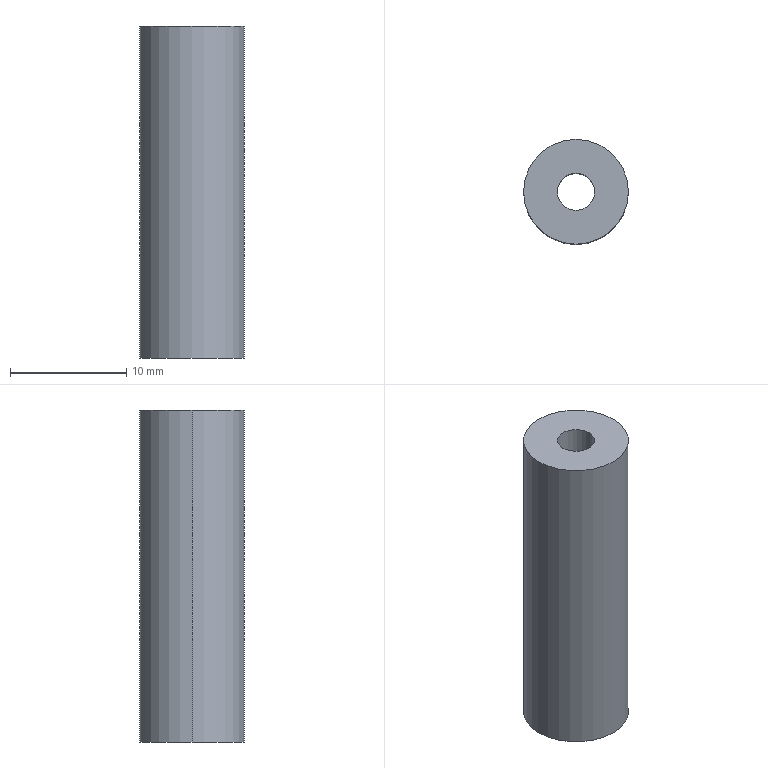Part | SolidWorks | features Extrusion 1 | 1 solid | 6 faces | box 9 x 9 x 28.5 mm | volume 1584 mm3 | cylinder 4 | plane 2 | commonest cylinder face diameters 3.2 x2 9 x2
STEP:
#1=CARTESIAN_POINT('',(-1.6,0.,14.25));
#2=VERTEX_POINT('',#1);
#3=CARTESIAN_POINT('',(1.6,0.,14.25));
#4=VERTEX_POINT('',#3);
#5=CARTESIAN_POINT('',(0.,0.,14.25));
#6=DIRECTION('',(0.,0.,1.));
#7=DIRECTION('',(1.,0.,0.));
#8=AXIS2_PLACEMENT_3D('',#5,#6,#7);
#9=CIRCLE('',#8,1.6);
#10=EDGE_CURVE('',#2,#4,#9,.T.);
#11=ORIENTED_EDGE('',*,*,#10,.T.);
#12=CARTESIAN_POINT('',(1.6,0.,-14.25));
#13=VERTEX_POINT('',#12);
#14=CARTESIAN_POINT('',(1.6,0.,14.25));
#15=DIRECTION('',(0.,0.,-1.));
#16=VECTOR('',#15,1000.);
#17=LINE('',#14,#16);
#18=EDGE_CURVE('',#4,#13,#17,.T.);
#19=ORIENTED_EDGE('',*,*,#18,.T.);
#20=CARTESIAN_POINT('',(-1.6,0.,-14.25));
#21=VERTEX_POINT('',#20);
#22=CARTESIAN_POINT('',(0.,0.,-14.25));
#23=DIRECTION('',(0.,0.,1.));
#24=DIRECTION('',(1.,0.,0.));
#25=AXIS2_PLACEMENT_3D('',#22,#23,#24);
#26=CIRCLE('',#25,1.6);
#27=EDGE_CURVE('',#21,#13,#26,.T.);
#28=ORIENTED_EDGE('',*,*,#27,.F.);
#29=CARTESIAN_POINT('',(-1.6,0.,14.25));
#30=DIRECTION('',(0.,0.,-1.));
#31=VECTOR('',#30,1000.);
#32=LINE('',#29,#31);
#33=EDGE_CURVE('',#2,#21,#32,.T.);
#34=ORIENTED_EDGE('',*,*,#33,.F.);
#35=EDGE_LOOP('',(#11,#19,#28,#34));
#36=FACE_OUTER_BOUND('',#35,.T.);
#37=CARTESIAN_POINT('',(0.,0.,14.25));
#38=DIRECTION('',(0.,0.,-1.));
#39=DIRECTION('',(-1.,0.,0.));
#40=AXIS2_PLACEMENT_3D('',#37,#38,#39);
#41=CYLINDRICAL_SURFACE('',#40,1.6);
#42=ADVANCED_FACE('',(#36),#41,.F.);
#43=CARTESIAN_POINT('',(4.5,0.,14.25));
#44=VERTEX_POINT('',#43);
#45=CARTESIAN_POINT('',(-4.5,0.,14.25));
#46=VERTEX_POINT('',#45);
#47=CARTESIAN_POINT('',(0.,0.,14.25));
#48=DIRECTION('',(0.,0.,1.));
#49=DIRECTION('',(1.,0.,0.));
#50=AXIS2_PLACEMENT_3D('',#47,#48,#49);
#51=CIRCLE('',#50,4.5);
#52=EDGE_CURVE('',#44,#46,#51,.T.);
#53=ORIENTED_EDGE('',*,*,#52,.F.);
#54=CARTESIAN_POINT('',(4.5,0.,-14.25));
#55=VERTEX_POINT('',#54);
#56=CARTESIAN_POINT('',(4.5,0.,14.25));
#57=DIRECTION('',(0.,0.,-1.));
#58=VECTOR('',#57,1000.);
#59=LINE('',#56,#58);
#60=EDGE_CURVE('',#44,#55,#59,.T.);
#61=ORIENTED_EDGE('',*,*,#60,.T.);
#62=CARTESIAN_POINT('',(-4.5,0.,-14.25));
#63=VERTEX_POINT('',#62);
#64=CARTESIAN_POINT('',(0.,0.,-14.25));
#65=DIRECTION('',(0.,0.,1.));
#66=DIRECTION('',(1.,0.,0.));
#67=AXIS2_PLACEMENT_3D('',#64,#65,#66);
#68=CIRCLE('',#67,4.5);
#69=EDGE_CURVE('',#55,#63,#68,.T.);
#70=ORIENTED_EDGE('',*,*,#69,.T.);
#71=CARTESIAN_POINT('',(-4.5,0.,14.25));
#72=DIRECTION('',(0.,0.,-1.));
#73=VECTOR('',#72,1000.);
#74=LINE('',#71,#73);
#75=EDGE_CURVE('',#46,#63,#74,.T.);
#76=ORIENTED_EDGE('',*,*,#75,.F.);
#77=EDGE_LOOP('',(#53,#61,#70,#76));
#78=FACE_OUTER_BOUND('',#77,.T.);
#79=CARTESIAN_POINT('',(0.,0.,14.25));
#80=DIRECTION('',(0.,0.,-1.));
#81=DIRECTION('',(-1.,0.,0.));
#82=AXIS2_PLACEMENT_3D('',#79,#80,#81);
#83=CYLINDRICAL_SURFACE('',#82,4.5);
#84=ADVANCED_FACE('',(#78),#83,.T.);
#85=CARTESIAN_POINT('',(0.,0.,14.25));
#86=DIRECTION('',(0.,0.,1.));
#87=DIRECTION('',(1.,0.,0.));
#88=AXIS2_PLACEMENT_3D('',#85,#86,#87);
#89=CIRCLE('',#88,4.5);
#90=EDGE_CURVE('',#46,#44,#89,.T.);
#91=ORIENTED_EDGE('',*,*,#90,.T.);
#92=ORIENTED_EDGE('',*,*,#52,.T.);
#93=EDGE_LOOP('',(#91,#92));
#94=FACE_OUTER_BOUND('',#93,.T.);
#95=ORIENTED_EDGE('',*,*,#10,.F.);
#96=CARTESIAN_POINT('',(0.,0.,14.25));
#97=DIRECTION('',(0.,0.,1.));
#98=DIRECTION('',(1.,0.,0.));
#99=AXIS2_PLACEMENT_3D('',#96,#97,#98);
#100=CIRCLE('',#99,1.6);
#101=EDGE_CURVE('',#4,#2,#100,.T.);
#102=ORIENTED_EDGE('',*,*,#101,.F.);
#103=EDGE_LOOP('',(#95,#102));
#104=FACE_BOUND('',#103,.T.);
#105=CARTESIAN_POINT('',(0.,0.,14.25));
#106=DIRECTION('',(0.,0.,1.));
#107=DIRECTION('',(1.,0.,0.));
#108=AXIS2_PLACEMENT_3D('',#105,#106,#107);
#109=PLANE('',#108);
#110=ADVANCED_FACE('',(#94,#104),#109,.T.);
#111=CARTESIAN_POINT('',(0.,0.,-14.25));
#112=DIRECTION('',(0.,0.,1.));
#113=DIRECTION('',(1.,0.,0.));
#114=AXIS2_PLACEMENT_3D('',#111,#112,#113);
#115=CIRCLE('',#114,4.5);
#116=EDGE_CURVE('',#63,#55,#115,.T.);
#117=ORIENTED_EDGE('',*,*,#116,.F.);
#118=ORIENTED_EDGE('',*,*,#69,.F.);
#119=EDGE_LOOP('',(#117,#118));
#120=FACE_OUTER_BOUND('',#119,.T.);
#121=ORIENTED_EDGE('',*,*,#27,.T.);
#122=CARTESIAN_POINT('',(0.,0.,-14.25));
#123=DIRECTION('',(0.,0.,1.));
#124=DIRECTION('',(1.,0.,0.));
#125=AXIS2_PLACEMENT_3D('',#122,#123,#124);
#126=CIRCLE('',#125,1.6);
#127=EDGE_CURVE('',#13,#21,#126,.T.);
#128=ORIENTED_EDGE('',*,*,#127,.T.);
#129=EDGE_LOOP('',(#121,#128));
#130=FACE_BOUND('',#129,.T.);
#131=CARTESIAN_POINT('',(0.,0.,-14.25));
#132=DIRECTION('',(0.,0.,1.));
#133=DIRECTION('',(1.,0.,0.));
#134=AXIS2_PLACEMENT_3D('',#131,#132,#133);
#135=PLANE('',#134);
#136=ADVANCED_FACE('',(#120,#130),#135,.F.);
#137=ORIENTED_EDGE('',*,*,#60,.F.);
#138=ORIENTED_EDGE('',*,*,#90,.F.);
#139=ORIENTED_EDGE('',*,*,#75,.T.);
#140=ORIENTED_EDGE('',*,*,#116,.T.);
#141=EDGE_LOOP('',(#137,#138,#139,#140));
#142=FACE_OUTER_BOUND('',#141,.T.);
#143=CARTESIAN_POINT('',(0.,0.,14.25));
#144=DIRECTION('',(0.,0.,-1.));
#145=DIRECTION('',(-1.,0.,0.));
#146=AXIS2_PLACEMENT_3D('',#143,#144,#145);
#147=CYLINDRICAL_SURFACE('',#146,4.5);
#148=ADVANCED_FACE('',(#142),#147,.T.);
#149=ORIENTED_EDGE('',*,*,#18,.F.);
#150=ORIENTED_EDGE('',*,*,#101,.T.);
#151=ORIENTED_EDGE('',*,*,#33,.T.);
#152=ORIENTED_EDGE('',*,*,#127,.F.);
#153=EDGE_LOOP('',(#149,#150,#151,#152));
#154=FACE_OUTER_BOUND('',#153,.T.);
#155=CARTESIAN_POINT('',(0.,0.,14.25));
#156=DIRECTION('',(0.,0.,-1.));
#157=DIRECTION('',(-1.,0.,0.));
#158=AXIS2_PLACEMENT_3D('',#155,#156,#157);
#159=CYLINDRICAL_SURFACE('',#158,1.6);
#160=ADVANCED_FACE('',(#154),#159,.F.);
#161=CLOSED_SHELL('',(#42,#84,#110,#136,#148,#160));
#162=MANIFOLD_SOLID_BREP('',#161);
#163=CARTESIAN_POINT('',(0.,0.,0.));
#164=DIRECTION('',(0.,0.,1.));
#165=DIRECTION('',(1.,0.,0.));
#166=AXIS2_PLACEMENT_3D('',#163,#164,#165);
#167=(LENGTH_UNIT()NAMED_UNIT(*)SI_UNIT(.MILLI.,.METRE.));
#168=UNCERTAINTY_MEASURE_WITH_UNIT(LENGTH_MEASURE(0.00001),#167,'','');
#169=(NAMED_UNIT(*)PLANE_ANGLE_UNIT()SI_UNIT($,.RADIAN.));
#170=(NAMED_UNIT(*)SI_UNIT($,.STERADIAN.)SOLID_ANGLE_UNIT());
#171=(GEOMETRIC_REPRESENTATION_CONTEXT(3)GLOBAL_UNCERTAINTY_ASSIGNED_CONTEXT((#168))GLOBAL_UNIT_ASSIGNED_CONTEXT((#167,#169,#170))REPRESENTATION_CONTEXT('',''));
#172=ADVANCED_BREP_SHAPE_REPRESENTATION('',(#162,#166),#171);